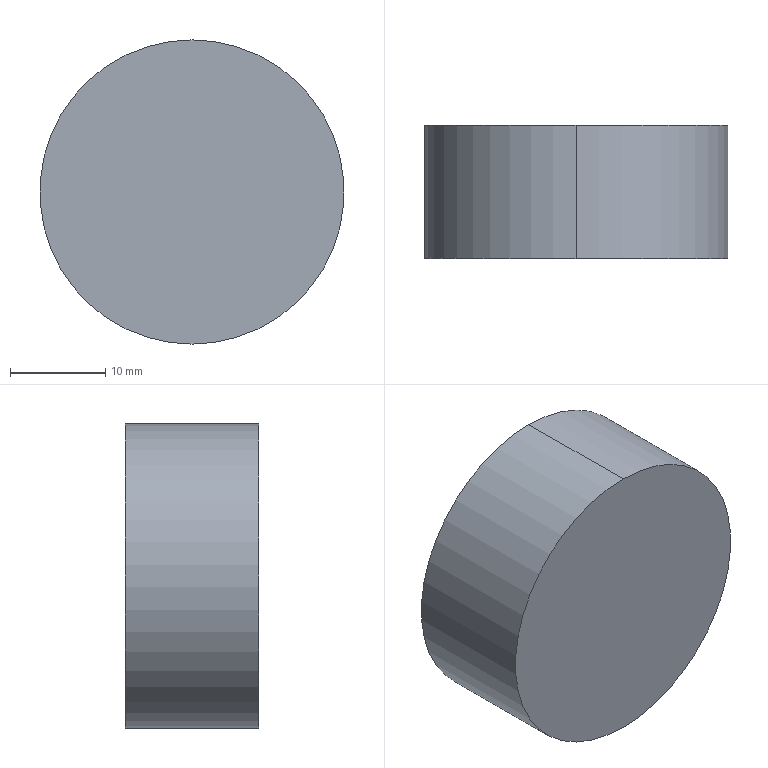Part | SolidWorks | features Extrusion 1 | 1 solid | 4 faces | box 32 x 14 x 32 mm | volume 11259 mm3 | cylinder 2 | plane 2 | commonest cylinder face diameters 32 x2
STEP:
#1=CARTESIAN_POINT('',(0.,14.,16.));
#2=VERTEX_POINT('',#1);
#3=CARTESIAN_POINT('',(0.,14.,-16.));
#4=VERTEX_POINT('',#3);
#5=CARTESIAN_POINT('',(0.,14.,0.));
#6=DIRECTION('',(0.,1.,0.));
#7=DIRECTION('',(0.,0.,1.));
#8=AXIS2_PLACEMENT_3D('',#5,#6,#7);
#9=CIRCLE('',#8,16.);
#10=EDGE_CURVE('',#2,#4,#9,.T.);
#11=ORIENTED_EDGE('',*,*,#10,.F.);
#12=CARTESIAN_POINT('',(0.,0.,16.));
#13=VERTEX_POINT('',#12);
#14=CARTESIAN_POINT('',(0.,14.,16.));
#15=DIRECTION('',(0.,-1.,0.));
#16=VECTOR('',#15,1000.);
#17=LINE('',#14,#16);
#18=EDGE_CURVE('',#2,#13,#17,.T.);
#19=ORIENTED_EDGE('',*,*,#18,.T.);
#20=CARTESIAN_POINT('',(0.,0.,-16.));
#21=VERTEX_POINT('',#20);
#22=CARTESIAN_POINT('',(0.,0.,0.));
#23=DIRECTION('',(0.,1.,0.));
#24=DIRECTION('',(0.,0.,1.));
#25=AXIS2_PLACEMENT_3D('',#22,#23,#24);
#26=CIRCLE('',#25,16.);
#27=EDGE_CURVE('',#13,#21,#26,.T.);
#28=ORIENTED_EDGE('',*,*,#27,.T.);
#29=CARTESIAN_POINT('',(0.,14.,-16.));
#30=DIRECTION('',(0.,-1.,0.));
#31=VECTOR('',#30,1000.);
#32=LINE('',#29,#31);
#33=EDGE_CURVE('',#4,#21,#32,.T.);
#34=ORIENTED_EDGE('',*,*,#33,.F.);
#35=EDGE_LOOP('',(#11,#19,#28,#34));
#36=FACE_OUTER_BOUND('',#35,.T.);
#37=CARTESIAN_POINT('',(0.,14.,0.));
#38=DIRECTION('',(0.,-1.,0.));
#39=DIRECTION('',(0.,0.,-1.));
#40=AXIS2_PLACEMENT_3D('',#37,#38,#39);
#41=CYLINDRICAL_SURFACE('',#40,16.);
#42=ADVANCED_FACE('',(#36),#41,.T.);
#43=ORIENTED_EDGE('',*,*,#18,.F.);
#44=CARTESIAN_POINT('',(0.,14.,0.));
#45=DIRECTION('',(0.,1.,0.));
#46=DIRECTION('',(0.,0.,1.));
#47=AXIS2_PLACEMENT_3D('',#44,#45,#46);
#48=CIRCLE('',#47,16.);
#49=EDGE_CURVE('',#4,#2,#48,.T.);
#50=ORIENTED_EDGE('',*,*,#49,.F.);
#51=ORIENTED_EDGE('',*,*,#33,.T.);
#52=CARTESIAN_POINT('',(0.,0.,0.));
#53=DIRECTION('',(0.,1.,0.));
#54=DIRECTION('',(0.,0.,1.));
#55=AXIS2_PLACEMENT_3D('',#52,#53,#54);
#56=CIRCLE('',#55,16.);
#57=EDGE_CURVE('',#21,#13,#56,.T.);
#58=ORIENTED_EDGE('',*,*,#57,.T.);
#59=EDGE_LOOP('',(#43,#50,#51,#58));
#60=FACE_OUTER_BOUND('',#59,.T.);
#61=CARTESIAN_POINT('',(0.,14.,0.));
#62=DIRECTION('',(0.,-1.,0.));
#63=DIRECTION('',(0.,0.,-1.));
#64=AXIS2_PLACEMENT_3D('',#61,#62,#63);
#65=CYLINDRICAL_SURFACE('',#64,16.);
#66=ADVANCED_FACE('',(#60),#65,.T.);
#67=ORIENTED_EDGE('',*,*,#49,.T.);
#68=ORIENTED_EDGE('',*,*,#10,.T.);
#69=EDGE_LOOP('',(#67,#68));
#70=FACE_OUTER_BOUND('',#69,.T.);
#71=CARTESIAN_POINT('',(0.,14.,0.));
#72=DIRECTION('',(0.,1.,0.));
#73=DIRECTION('',(0.,0.,1.));
#74=AXIS2_PLACEMENT_3D('',#71,#72,#73);
#75=PLANE('',#74);
#76=ADVANCED_FACE('',(#70),#75,.T.);
#77=ORIENTED_EDGE('',*,*,#57,.F.);
#78=ORIENTED_EDGE('',*,*,#27,.F.);
#79=EDGE_LOOP('',(#77,#78));
#80=FACE_OUTER_BOUND('',#79,.T.);
#81=CARTESIAN_POINT('',(0.,0.,0.));
#82=DIRECTION('',(0.,1.,0.));
#83=DIRECTION('',(0.,0.,1.));
#84=AXIS2_PLACEMENT_3D('',#81,#82,#83);
#85=PLANE('',#84);
#86=ADVANCED_FACE('',(#80),#85,.F.);
#87=CLOSED_SHELL('',(#42,#66,#76,#86));
#88=MANIFOLD_SOLID_BREP('',#87);
#89=CARTESIAN_POINT('',(0.,0.,0.));
#90=DIRECTION('',(0.,0.,1.));
#91=DIRECTION('',(1.,0.,0.));
#92=AXIS2_PLACEMENT_3D('',#89,#90,#91);
#93=(LENGTH_UNIT()NAMED_UNIT(*)SI_UNIT(.MILLI.,.METRE.));
#94=UNCERTAINTY_MEASURE_WITH_UNIT(LENGTH_MEASURE(0.00001),#93,'','');
#95=(NAMED_UNIT(*)PLANE_ANGLE_UNIT()SI_UNIT($,.RADIAN.));
#96=(NAMED_UNIT(*)SI_UNIT($,.STERADIAN.)SOLID_ANGLE_UNIT());
#97=(GEOMETRIC_REPRESENTATION_CONTEXT(3)GLOBAL_UNCERTAINTY_ASSIGNED_CONTEXT((#94))GLOBAL_UNIT_ASSIGNED_CONTEXT((#93,#95,#96))REPRESENTATION_CONTEXT('',''));
#98=ADVANCED_BREP_SHAPE_REPRESENTATION('',(#88,#92),#97);